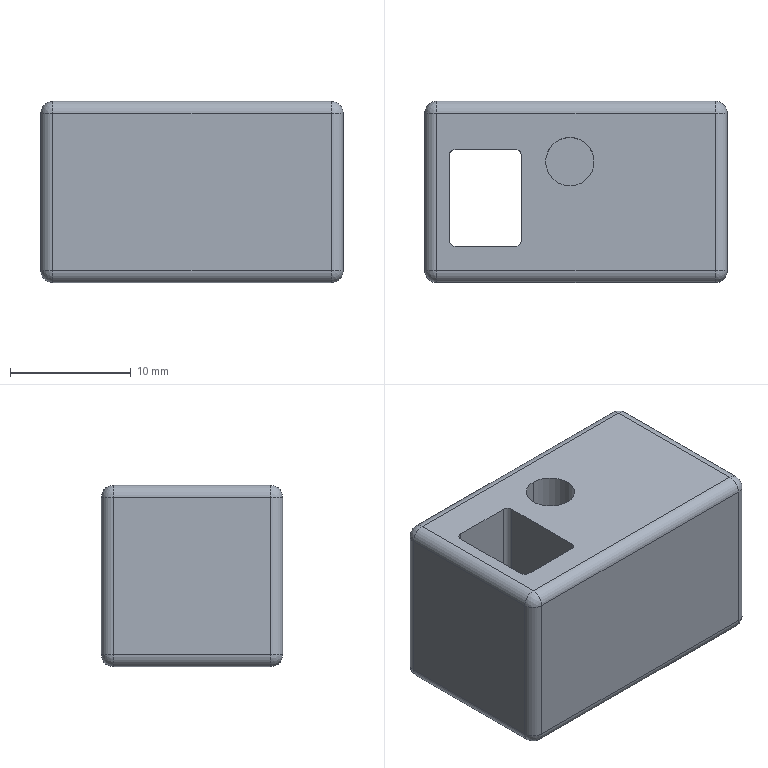Part | NX | 1 solid | 40 faces | box 25 x 15 x 15 mm | volume 4703 mm3 | cylinder 20 | plane 12 | sphere 8 | commonest cylinder face diameters 2 x12 1 x4 3.5 x2 4 x2
STEP:
#1=CARTESIAN_POINT('',(12.5,-6.5,-14.));
#2=VERTEX_POINT('',#1);
#3=CARTESIAN_POINT('',(12.5,6.5,-14.));
#4=VERTEX_POINT('',#3);
#5=CARTESIAN_POINT('',(12.5,-6.5,-14.));
#6=DIRECTION('',(0.,1.,0.));
#7=VECTOR('',#6,1000.);
#8=LINE('',#5,#7);
#9=EDGE_CURVE('',#2,#4,#8,.T.);
#10=ORIENTED_EDGE('',*,*,#9,.T.);
#11=CARTESIAN_POINT('',(12.5,6.5,-1.));
#12=VERTEX_POINT('',#11);
#13=CARTESIAN_POINT('',(12.5,6.5,-14.));
#14=DIRECTION('',(0.,0.,1.));
#15=VECTOR('',#14,1000.);
#16=LINE('',#13,#15);
#17=EDGE_CURVE('',#4,#12,#16,.T.);
#18=ORIENTED_EDGE('',*,*,#17,.T.);
#19=CARTESIAN_POINT('',(12.5,-6.5,-1.));
#20=VERTEX_POINT('',#19);
#21=CARTESIAN_POINT('',(12.5,6.5,-1.));
#22=DIRECTION('',(0.,-1.,0.));
#23=VECTOR('',#22,1000.);
#24=LINE('',#21,#23);
#25=EDGE_CURVE('',#12,#20,#24,.T.);
#26=ORIENTED_EDGE('',*,*,#25,.T.);
#27=CARTESIAN_POINT('',(12.5,-6.5,-1.));
#28=DIRECTION('',(0.,0.,-1.));
#29=VECTOR('',#28,1000.);
#30=LINE('',#27,#29);
#31=EDGE_CURVE('',#20,#2,#30,.T.);
#32=ORIENTED_EDGE('',*,*,#31,.T.);
#33=EDGE_LOOP('',(#10,#18,#26,#32));
#34=FACE_BOUND('',#33,.T.);
#35=CARTESIAN_POINT('',(12.5,0.75,-7.5));
#36=VERTEX_POINT('',#35);
#37=CARTESIAN_POINT('',(12.5,4.25,-7.5));
#38=VERTEX_POINT('',#37);
#39=CARTESIAN_POINT('',(12.5,2.5,-7.5));
#40=DIRECTION('',(1.,0.,0.));
#41=DIRECTION('',(0.,-1.,0.));
#42=AXIS2_PLACEMENT_3D('',#39,#40,#41);
#43=CIRCLE('',#42,1.75);
#44=EDGE_CURVE('',#36,#38,#43,.T.);
#45=ORIENTED_EDGE('',*,*,#44,.F.);
#46=CARTESIAN_POINT('',(12.5,2.5,-7.5));
#47=DIRECTION('',(1.,0.,0.));
#48=DIRECTION('',(0.,1.,0.));
#49=AXIS2_PLACEMENT_3D('',#46,#47,#48);
#50=CIRCLE('',#49,1.75);
#51=EDGE_CURVE('',#38,#36,#50,.T.);
#52=ORIENTED_EDGE('',*,*,#51,.F.);
#53=EDGE_LOOP('',(#45,#52));
#54=FACE_BOUND('',#53,.T.);
#55=CARTESIAN_POINT('',(12.5,-26.5,-53.));
#56=DIRECTION('',(-1.,0.,0.));
#57=DIRECTION('',(0.,1.,0.));
#58=AXIS2_PLACEMENT_3D('',#55,#56,#57);
#59=PLANE('',#58);
#60=ADVANCED_FACE('',(#34,#54),#59,.F.);
#61=CARTESIAN_POINT('',(2.5,0.75,-7.5));
#62=VERTEX_POINT('',#61);
#63=CARTESIAN_POINT('',(12.5,0.75,-7.5));
#64=DIRECTION('',(-1.,0.,0.));
#65=VECTOR('',#64,1000.);
#66=LINE('',#63,#65);
#67=EDGE_CURVE('',#36,#62,#66,.T.);
#68=ORIENTED_EDGE('',*,*,#67,.T.);
#69=CARTESIAN_POINT('',(2.5,4.25,-7.5));
#70=VERTEX_POINT('',#69);
#71=CARTESIAN_POINT('',(2.5,2.5,-7.5));
#72=DIRECTION('',(1.,0.,0.));
#73=DIRECTION('',(0.,1.,0.));
#74=AXIS2_PLACEMENT_3D('',#71,#72,#73);
#75=CIRCLE('',#74,1.75);
#76=EDGE_CURVE('',#70,#62,#75,.T.);
#77=ORIENTED_EDGE('',*,*,#76,.F.);
#78=CARTESIAN_POINT('',(12.5,4.25,-7.5));
#79=DIRECTION('',(-1.,0.,0.));
#80=VECTOR('',#79,1000.);
#81=LINE('',#78,#80);
#82=EDGE_CURVE('',#38,#70,#81,.T.);
#83=ORIENTED_EDGE('',*,*,#82,.F.);
#84=ORIENTED_EDGE('',*,*,#51,.T.);
#85=EDGE_LOOP('',(#68,#77,#83,#84));
#86=FACE_BOUND('',#85,.T.);
#87=CARTESIAN_POINT('',(12.5,2.5,-7.5));
#88=DIRECTION('',(1.,0.,0.));
#89=DIRECTION('',(0.,-1.,0.));
#90=AXIS2_PLACEMENT_3D('',#87,#88,#89);
#91=CYLINDRICAL_SURFACE('',#90,1.75);
#92=ADVANCED_FACE('',(#86),#91,.F.);
#93=ORIENTED_EDGE('',*,*,#82,.T.);
#94=CARTESIAN_POINT('',(2.5,2.5,-7.5));
#95=DIRECTION('',(1.,0.,0.));
#96=DIRECTION('',(0.,-1.,0.));
#97=AXIS2_PLACEMENT_3D('',#94,#95,#96);
#98=CIRCLE('',#97,1.75);
#99=EDGE_CURVE('',#62,#70,#98,.T.);
#100=ORIENTED_EDGE('',*,*,#99,.F.);
#101=ORIENTED_EDGE('',*,*,#67,.F.);
#102=ORIENTED_EDGE('',*,*,#44,.T.);
#103=EDGE_LOOP('',(#93,#100,#101,#102));
#104=FACE_BOUND('',#103,.T.);
#105=CARTESIAN_POINT('',(12.5,2.5,-7.5));
#106=DIRECTION('',(1.,0.,0.));
#107=DIRECTION('',(0.,-1.,0.));
#108=AXIS2_PLACEMENT_3D('',#105,#106,#107);
#109=CYLINDRICAL_SURFACE('',#108,1.75);
#110=ADVANCED_FACE('',(#104),#109,.F.);
#111=ORIENTED_EDGE('',*,*,#99,.T.);
#112=ORIENTED_EDGE('',*,*,#76,.T.);
#113=EDGE_LOOP('',(#111,#112));
#114=FACE_BOUND('',#113,.T.);
#115=CARTESIAN_POINT('',(2.5,-26.5,-53.));
#116=DIRECTION('',(1.,0.,0.));
#117=DIRECTION('',(0.,-1.,0.));
#118=AXIS2_PLACEMENT_3D('',#115,#116,#117);
#119=PLANE('',#118);
#120=ADVANCED_FACE('',(#114),#119,.T.);
#121=CARTESIAN_POINT('',(11.5,-7.5,-1.));
#122=VERTEX_POINT('',#121);
#123=CARTESIAN_POINT('',(11.5,-6.5,-1.));
#124=DIRECTION('',(0.,0.,-1.));
#125=DIRECTION('',(1.,0.,0.));
#126=AXIS2_PLACEMENT_3D('',#123,#124,#125);
#127=CIRCLE('',#126,1.);
#128=EDGE_CURVE('',#20,#122,#127,.T.);
#129=ORIENTED_EDGE('',*,*,#128,.T.);
#130=CARTESIAN_POINT('',(11.5,-7.5,-14.));
#131=VERTEX_POINT('',#130);
#132=CARTESIAN_POINT('',(11.5,-7.5,-1.));
#133=DIRECTION('',(0.,0.,-1.));
#134=VECTOR('',#133,1000.);
#135=LINE('',#132,#134);
#136=EDGE_CURVE('',#122,#131,#135,.T.);
#137=ORIENTED_EDGE('',*,*,#136,.T.);
#138=CARTESIAN_POINT('',(11.5,-6.5,-14.));
#139=DIRECTION('',(0.,0.,-1.));
#140=DIRECTION('',(1.,0.,0.));
#141=AXIS2_PLACEMENT_3D('',#138,#139,#140);
#142=CIRCLE('',#141,1.);
#143=EDGE_CURVE('',#2,#131,#142,.T.);
#144=ORIENTED_EDGE('',*,*,#143,.F.);
#145=ORIENTED_EDGE('',*,*,#31,.F.);
#146=EDGE_LOOP('',(#129,#137,#144,#145));
#147=FACE_BOUND('',#146,.T.);
#148=CARTESIAN_POINT('',(11.5,-6.5,-0.9345));
#149=DIRECTION('',(0.,0.,-1.));
#150=DIRECTION('',(-1.,0.,0.));
#151=AXIS2_PLACEMENT_3D('',#148,#149,#150);
#152=CYLINDRICAL_SURFACE('',#151,1.);
#153=ADVANCED_FACE('',(#147),#152,.T.);
#154=ORIENTED_EDGE('',*,*,#143,.T.);
#155=CARTESIAN_POINT('',(11.5,-6.5,-15.));
#156=VERTEX_POINT('',#155);
#157=CARTESIAN_POINT('',(11.5,-6.5,-14.));
#158=DIRECTION('',(-1.,0.,0.));
#159=DIRECTION('',(0.,0.,-1.));
#160=AXIS2_PLACEMENT_3D('',#157,#158,#159);
#161=CIRCLE('',#160,1.);
#162=EDGE_CURVE('',#156,#131,#161,.T.);
#163=ORIENTED_EDGE('',*,*,#162,.F.);
#164=CARTESIAN_POINT('',(11.5,-6.5,-14.));
#165=DIRECTION('',(0.,1.,0.));
#166=DIRECTION('',(1.,0.,0.));
#167=AXIS2_PLACEMENT_3D('',#164,#165,#166);
#168=CIRCLE('',#167,1.);
#169=EDGE_CURVE('',#2,#156,#168,.T.);
#170=ORIENTED_EDGE('',*,*,#169,.F.);
#171=EDGE_LOOP('',(#154,#163,#170));
#172=FACE_BOUND('',#171,.T.);
#173=CARTESIAN_POINT('',(11.5,-6.5,-14.));
#174=DIRECTION('',(0.7071,0.,0.7071));
#175=DIRECTION('',(-0.7071,0.,0.7071));
#176=AXIS2_PLACEMENT_3D('',#173,#174,#175);
#177=SPHERICAL_SURFACE('',#176,1.);
#178=ADVANCED_FACE('',(#172),#177,.T.);
#179=CARTESIAN_POINT('',(11.5,6.5,-15.));
#180=VERTEX_POINT('',#179);
#181=CARTESIAN_POINT('',(11.5,-6.5,-15.));
#182=DIRECTION('',(0.,1.,0.));
#183=VECTOR('',#182,1000.);
#184=LINE('',#181,#183);
#185=EDGE_CURVE('',#156,#180,#184,.T.);
#186=ORIENTED_EDGE('',*,*,#185,.T.);
#187=CARTESIAN_POINT('',(11.5,6.5,-14.));
#188=DIRECTION('',(0.,-1.,0.));
#189=DIRECTION('',(0.,0.,-1.));
#190=AXIS2_PLACEMENT_3D('',#187,#188,#189);
#191=CIRCLE('',#190,1.);
#192=EDGE_CURVE('',#180,#4,#191,.T.);
#193=ORIENTED_EDGE('',*,*,#192,.T.);
#194=ORIENTED_EDGE('',*,*,#9,.F.);
#195=ORIENTED_EDGE('',*,*,#169,.T.);
#196=EDGE_LOOP('',(#186,#193,#194,#195));
#197=FACE_BOUND('',#196,.T.);
#198=CARTESIAN_POINT('',(11.5,-11.591,-14.));
#199=DIRECTION('',(0.,1.,0.));
#200=DIRECTION('',(-1.,0.,0.));
#201=AXIS2_PLACEMENT_3D('',#198,#199,#200);
#202=CYLINDRICAL_SURFACE('',#201,1.);
#203=ADVANCED_FACE('',(#197),#202,.T.);
#204=CARTESIAN_POINT('',(11.5,7.5,-14.));
#205=VERTEX_POINT('',#204);
#206=CARTESIAN_POINT('',(11.5,6.5,-14.));
#207=DIRECTION('',(1.,0.,0.));
#208=DIRECTION('',(0.,0.,-1.));
#209=AXIS2_PLACEMENT_3D('',#206,#207,#208);
#210=CIRCLE('',#209,1.);
#211=EDGE_CURVE('',#180,#205,#210,.T.);
#212=ORIENTED_EDGE('',*,*,#211,.T.);
#213=CARTESIAN_POINT('',(11.5,6.5,-14.));
#214=DIRECTION('',(0.,0.,1.));
#215=DIRECTION('',(1.,0.,0.));
#216=AXIS2_PLACEMENT_3D('',#213,#214,#215);
#217=CIRCLE('',#216,1.);
#218=EDGE_CURVE('',#4,#205,#217,.T.);
#219=ORIENTED_EDGE('',*,*,#218,.F.);
#220=ORIENTED_EDGE('',*,*,#192,.F.);
#221=EDGE_LOOP('',(#212,#219,#220));
#222=FACE_BOUND('',#221,.T.);
#223=CARTESIAN_POINT('',(11.5,6.5,-14.));
#224=DIRECTION('',(-0.7071,0.,-0.7071));
#225=DIRECTION('',(-0.7071,0.,0.7071));
#226=AXIS2_PLACEMENT_3D('',#223,#224,#225);
#227=SPHERICAL_SURFACE('',#226,1.);
#228=ADVANCED_FACE('',(#222),#227,.T.);
#229=ORIENTED_EDGE('',*,*,#218,.T.);
#230=CARTESIAN_POINT('',(11.5,7.5,-1.));
#231=VERTEX_POINT('',#230);
#232=CARTESIAN_POINT('',(11.5,7.5,-14.));
#233=DIRECTION('',(0.,0.,1.));
#234=VECTOR('',#233,1000.);
#235=LINE('',#232,#234);
#236=EDGE_CURVE('',#205,#231,#235,.T.);
#237=ORIENTED_EDGE('',*,*,#236,.T.);
#238=CARTESIAN_POINT('',(11.5,6.5,-1.));
#239=DIRECTION('',(0.,0.,1.));
#240=DIRECTION('',(1.,0.,0.));
#241=AXIS2_PLACEMENT_3D('',#238,#239,#240);
#242=CIRCLE('',#241,1.);
#243=EDGE_CURVE('',#12,#231,#242,.T.);
#244=ORIENTED_EDGE('',*,*,#243,.F.);
#245=ORIENTED_EDGE('',*,*,#17,.F.);
#246=EDGE_LOOP('',(#229,#237,#244,#245));
#247=FACE_BOUND('',#246,.T.);
#248=CARTESIAN_POINT('',(11.5,6.5,-14.063));
#249=DIRECTION('',(0.,0.,1.));
#250=DIRECTION('',(-1.,0.,0.));
#251=AXIS2_PLACEMENT_3D('',#248,#249,#250);
#252=CYLINDRICAL_SURFACE('',#251,1.);
#253=ADVANCED_FACE('',(#247),#252,.T.);
#254=ORIENTED_EDGE('',*,*,#243,.T.);
#255=CARTESIAN_POINT('',(11.5,6.5,0.));
#256=VERTEX_POINT('',#255);
#257=CARTESIAN_POINT('',(11.5,6.5,-1.));
#258=DIRECTION('',(-1.,0.,0.));
#259=DIRECTION('',(0.,0.,1.));
#260=AXIS2_PLACEMENT_3D('',#257,#258,#259);
#261=CIRCLE('',#260,1.);
#262=EDGE_CURVE('',#256,#231,#261,.T.);
#263=ORIENTED_EDGE('',*,*,#262,.F.);
#264=CARTESIAN_POINT('',(11.5,6.5,-1.));
#265=DIRECTION('',(0.,-1.,0.));
#266=DIRECTION('',(1.,0.,0.));
#267=AXIS2_PLACEMENT_3D('',#264,#265,#266);
#268=CIRCLE('',#267,1.);
#269=EDGE_CURVE('',#12,#256,#268,.T.);
#270=ORIENTED_EDGE('',*,*,#269,.F.);
#271=EDGE_LOOP('',(#254,#263,#270));
#272=FACE_BOUND('',#271,.T.);
#273=CARTESIAN_POINT('',(11.5,6.5,-1.));
#274=DIRECTION('',(0.7071,0.,-0.7071));
#275=DIRECTION('',(-0.7071,0.,-0.7071));
#276=AXIS2_PLACEMENT_3D('',#273,#274,#275);
#277=SPHERICAL_SURFACE('',#276,1.);
#278=ADVANCED_FACE('',(#272),#277,.T.);
#279=ORIENTED_EDGE('',*,*,#25,.F.);
#280=ORIENTED_EDGE('',*,*,#269,.T.);
#281=CARTESIAN_POINT('',(11.5,-6.5,0.));
#282=VERTEX_POINT('',#281);
#283=CARTESIAN_POINT('',(11.5,6.5,0.));
#284=DIRECTION('',(0.,-1.,0.));
#285=VECTOR('',#284,1000.);
#286=LINE('',#283,#285);
#287=EDGE_CURVE('',#256,#282,#286,.T.);
#288=ORIENTED_EDGE('',*,*,#287,.T.);
#289=CARTESIAN_POINT('',(11.5,-6.5,-1.));
#290=DIRECTION('',(0.,1.,0.));
#291=DIRECTION('',(0.,0.,1.));
#292=AXIS2_PLACEMENT_3D('',#289,#290,#291);
#293=CIRCLE('',#292,1.);
#294=EDGE_CURVE('',#282,#20,#293,.T.);
#295=ORIENTED_EDGE('',*,*,#294,.T.);
#296=EDGE_LOOP('',(#279,#280,#288,#295));
#297=FACE_BOUND('',#296,.T.);
#298=CARTESIAN_POINT('',(11.5,16.591,-1.));
#299=DIRECTION('',(0.,-1.,0.));
#300=DIRECTION('',(-1.,0.,0.));
#301=AXIS2_PLACEMENT_3D('',#298,#299,#300);
#302=CYLINDRICAL_SURFACE('',#301,1.);
#303=ADVANCED_FACE('',(#297),#302,.T.);
#304=CARTESIAN_POINT('',(11.5,-6.5,-1.));
#305=DIRECTION('',(1.,0.,0.));
#306=DIRECTION('',(0.,0.,1.));
#307=AXIS2_PLACEMENT_3D('',#304,#305,#306);
#308=CIRCLE('',#307,1.);
#309=EDGE_CURVE('',#282,#122,#308,.T.);
#310=ORIENTED_EDGE('',*,*,#309,.T.);
#311=ORIENTED_EDGE('',*,*,#128,.F.);
#312=ORIENTED_EDGE('',*,*,#294,.F.);
#313=EDGE_LOOP('',(#310,#311,#312));
#314=FACE_BOUND('',#313,.T.);
#315=CARTESIAN_POINT('',(11.5,-6.5,-1.));
#316=DIRECTION('',(-0.7071,0.,0.7071));
#317=DIRECTION('',(-0.7071,0.,-0.7071));
#318=AXIS2_PLACEMENT_3D('',#315,#316,#317);
#319=SPHERICAL_SURFACE('',#318,1.);
#320=ADVANCED_FACE('',(#314),#319,.T.);
#321=CARTESIAN_POINT('',(-11.5,-6.5,0.));
#322=VERTEX_POINT('',#321);
#323=CARTESIAN_POINT('',(-11.5,-7.5,-1.));
#324=VERTEX_POINT('',#323);
#325=CARTESIAN_POINT('',(-11.5,-6.5,-1.));
#326=DIRECTION('',(1.,0.,0.));
#327=DIRECTION('',(0.,0.,1.));
#328=AXIS2_PLACEMENT_3D('',#325,#326,#327);
#329=CIRCLE('',#328,1.);
#330=EDGE_CURVE('',#322,#324,#329,.T.);
#331=ORIENTED_EDGE('',*,*,#330,.T.);
#332=CARTESIAN_POINT('',(-11.5,-7.5,-1.));
#333=DIRECTION('',(1.,0.,0.));
#334=VECTOR('',#333,1000.);
#335=LINE('',#332,#334);
#336=EDGE_CURVE('',#324,#122,#335,.T.);
#337=ORIENTED_EDGE('',*,*,#336,.T.);
#338=ORIENTED_EDGE('',*,*,#309,.F.);
#339=CARTESIAN_POINT('',(-11.5,-6.5,0.));
#340=DIRECTION('',(1.,0.,0.));
#341=VECTOR('',#340,1000.);
#342=LINE('',#339,#341);
#343=EDGE_CURVE('',#322,#282,#342,.T.);
#344=ORIENTED_EDGE('',*,*,#343,.F.);
#345=EDGE_LOOP('',(#331,#337,#338,#344));
#346=FACE_BOUND('',#345,.T.);
#347=CARTESIAN_POINT('',(-11.565,-6.5,-1.));
#348=DIRECTION('',(1.,0.,0.));
#349=DIRECTION('',(0.,0.,-1.));
#350=AXIS2_PLACEMENT_3D('',#347,#348,#349);
#351=CYLINDRICAL_SURFACE('',#350,1.);
#352=ADVANCED_FACE('',(#346),#351,.T.);
#353=ORIENTED_EDGE('',*,*,#287,.F.);
#354=CARTESIAN_POINT('',(-11.5,6.5,0.));
#355=VERTEX_POINT('',#354);
#356=CARTESIAN_POINT('',(11.5,6.5,0.));
#357=DIRECTION('',(-1.,0.,0.));
#358=VECTOR('',#357,1000.);
#359=LINE('',#356,#358);
#360=EDGE_CURVE('',#256,#355,#359,.T.);
#361=ORIENTED_EDGE('',*,*,#360,.T.);
#362=CARTESIAN_POINT('',(-11.5,-6.5,0.));
#363=DIRECTION('',(0.,1.,0.));
#364=VECTOR('',#363,1000.);
#365=LINE('',#362,#364);
#366=EDGE_CURVE('',#322,#355,#365,.T.);
#367=ORIENTED_EDGE('',*,*,#366,.F.);
#368=ORIENTED_EDGE('',*,*,#343,.T.);
#369=EDGE_LOOP('',(#353,#361,#367,#368));
#370=FACE_BOUND('',#369,.T.);
#371=CARTESIAN_POINT('',(-0.5,0.5,0.));
#372=VERTEX_POINT('',#371);
#373=CARTESIAN_POINT('',(-0.5,4.5,0.));
#374=VERTEX_POINT('',#373);
#375=CARTESIAN_POINT('',(-0.5,2.5,0.));
#376=DIRECTION('',(0.,0.,1.));
#377=DIRECTION('',(0.,-1.,0.));
#378=AXIS2_PLACEMENT_3D('',#375,#376,#377);
#379=CIRCLE('',#378,2.);
#380=EDGE_CURVE('',#372,#374,#379,.T.);
#381=ORIENTED_EDGE('',*,*,#380,.F.);
#382=CARTESIAN_POINT('',(-0.5,2.5,0.));
#383=DIRECTION('',(0.,0.,1.));
#384=DIRECTION('',(0.,1.,0.));
#385=AXIS2_PLACEMENT_3D('',#382,#383,#384);
#386=CIRCLE('',#385,2.);
#387=EDGE_CURVE('',#374,#372,#386,.T.);
#388=ORIENTED_EDGE('',*,*,#387,.F.);
#389=EDGE_LOOP('',(#381,#388));
#390=FACE_BOUND('',#389,.T.);
#391=CARTESIAN_POINT('',(-10.,-4.5,0.));
#392=VERTEX_POINT('',#391);
#393=CARTESIAN_POINT('',(-10.5,-4.,0.));
#394=VERTEX_POINT('',#393);
#395=CARTESIAN_POINT('',(-10.,-4.,0.));
#396=DIRECTION('',(0.,0.,-1.));
#397=DIRECTION('',(0.,-1.,0.));
#398=AXIS2_PLACEMENT_3D('',#395,#396,#397);
#399=CIRCLE('',#398,0.5);
#400=EDGE_CURVE('',#392,#394,#399,.T.);
#401=ORIENTED_EDGE('',*,*,#400,.T.);
#402=CARTESIAN_POINT('',(-10.5,3.,0.));
#403=VERTEX_POINT('',#402);
#404=CARTESIAN_POINT('',(-10.5,-4.,0.));
#405=DIRECTION('',(0.,1.,0.));
#406=VECTOR('',#405,1000.);
#407=LINE('',#404,#406);
#408=EDGE_CURVE('',#394,#403,#407,.T.);
#409=ORIENTED_EDGE('',*,*,#408,.T.);
#410=CARTESIAN_POINT('',(-10.,3.5,0.));
#411=VERTEX_POINT('',#410);
#412=CARTESIAN_POINT('',(-10.,3.,0.));
#413=DIRECTION('',(0.,0.,-1.));
#414=DIRECTION('',(-1.,0.,0.));
#415=AXIS2_PLACEMENT_3D('',#412,#413,#414);
#416=CIRCLE('',#415,0.5);
#417=EDGE_CURVE('',#403,#411,#416,.T.);
#418=ORIENTED_EDGE('',*,*,#417,.T.);
#419=CARTESIAN_POINT('',(-5.,3.5,0.));
#420=VERTEX_POINT('',#419);
#421=CARTESIAN_POINT('',(-10.,3.5,0.));
#422=DIRECTION('',(1.,0.,0.));
#423=VECTOR('',#422,1000.);
#424=LINE('',#421,#423);
#425=EDGE_CURVE('',#411,#420,#424,.T.);
#426=ORIENTED_EDGE('',*,*,#425,.T.);
#427=CARTESIAN_POINT('',(-4.5,3.,0.));
#428=VERTEX_POINT('',#427);
#429=CARTESIAN_POINT('',(-5.,3.,0.));
#430=DIRECTION('',(0.,0.,-1.));
#431=DIRECTION('',(0.,1.,0.));
#432=AXIS2_PLACEMENT_3D('',#429,#430,#431);
#433=CIRCLE('',#432,0.5);
#434=EDGE_CURVE('',#420,#428,#433,.T.);
#435=ORIENTED_EDGE('',*,*,#434,.T.);
#436=CARTESIAN_POINT('',(-4.5,-4.,0.));
#437=VERTEX_POINT('',#436);
#438=CARTESIAN_POINT('',(-4.5,3.,0.));
#439=DIRECTION('',(0.,-1.,0.));
#440=VECTOR('',#439,1000.);
#441=LINE('',#438,#440);
#442=EDGE_CURVE('',#428,#437,#441,.T.);
#443=ORIENTED_EDGE('',*,*,#442,.T.);
#444=CARTESIAN_POINT('',(-5.,-4.5,0.));
#445=VERTEX_POINT('',#444);
#446=CARTESIAN_POINT('',(-5.,-4.,0.));
#447=DIRECTION('',(0.,0.,-1.));
#448=DIRECTION('',(1.,0.,0.));
#449=AXIS2_PLACEMENT_3D('',#446,#447,#448);
#450=CIRCLE('',#449,0.5);
#451=EDGE_CURVE('',#437,#445,#450,.T.);
#452=ORIENTED_EDGE('',*,*,#451,.T.);
#453=CARTESIAN_POINT('',(-5.,-4.5,0.));
#454=DIRECTION('',(-1.,0.,0.));
#455=VECTOR('',#454,1000.);
#456=LINE('',#453,#455);
#457=EDGE_CURVE('',#445,#392,#456,.T.);
#458=ORIENTED_EDGE('',*,*,#457,.T.);
#459=EDGE_LOOP('',(#401,#409,#418,#426,#435,#443,#452,#458));
#460=FACE_BOUND('',#459,.T.);
#461=CARTESIAN_POINT('',(12.5,-12.5,0.));
#462=DIRECTION('',(0.,0.,1.));
#463=DIRECTION('',(0.,-1.,0.));
#464=AXIS2_PLACEMENT_3D('',#461,#462,#463);
#465=PLANE('',#464);
#466=ADVANCED_FACE('',(#370,#390,#460),#465,.T.);
#467=ORIENTED_EDGE('',*,*,#457,.F.);
#468=CARTESIAN_POINT('',(-5.,-4.5,-15.));
#469=VERTEX_POINT('',#468);
#470=CARTESIAN_POINT('',(-5.,-4.5,-15.));
#471=DIRECTION('',(0.,0.,1.));
#472=VECTOR('',#471,1000.);
#473=LINE('',#470,#472);
#474=EDGE_CURVE('',#469,#445,#473,.T.);
#475=ORIENTED_EDGE('',*,*,#474,.F.);
#476=CARTESIAN_POINT('',(-10.,-4.5,-15.));
#477=VERTEX_POINT('',#476);
#478=CARTESIAN_POINT('',(-5.,-4.5,-15.));
#479=DIRECTION('',(-1.,0.,0.));
#480=VECTOR('',#479,1000.);
#481=LINE('',#478,#480);
#482=EDGE_CURVE('',#469,#477,#481,.T.);
#483=ORIENTED_EDGE('',*,*,#482,.T.);
#484=CARTESIAN_POINT('',(-10.,-4.5,0.));
#485=DIRECTION('',(0.,0.,-1.));
#486=VECTOR('',#485,1000.);
#487=LINE('',#484,#486);
#488=EDGE_CURVE('',#392,#477,#487,.T.);
#489=ORIENTED_EDGE('',*,*,#488,.F.);
#490=EDGE_LOOP('',(#467,#475,#483,#489));
#491=FACE_BOUND('',#490,.T.);
#492=CARTESIAN_POINT('',(-2.5,-4.5,0.));
#493=DIRECTION('',(0.,1.,0.));
#494=DIRECTION('',(1.,0.,0.));
#495=AXIS2_PLACEMENT_3D('',#492,#493,#494);
#496=PLANE('',#495);
#497=ADVANCED_FACE('',(#491),#496,.T.);
#498=CARTESIAN_POINT('',(-10.5,-4.,-15.));
#499=VERTEX_POINT('',#498);
#500=CARTESIAN_POINT('',(-10.,-4.,-15.));
#501=DIRECTION('',(0.,0.,1.));
#502=DIRECTION('',(-1.,0.,0.));
#503=AXIS2_PLACEMENT_3D('',#500,#501,#502);
#504=CIRCLE('',#503,0.5);
#505=EDGE_CURVE('',#499,#477,#504,.T.);
#506=ORIENTED_EDGE('',*,*,#505,.F.);
#507=CARTESIAN_POINT('',(-10.5,-4.,0.));
#508=DIRECTION('',(0.,0.,-1.));
#509=VECTOR('',#508,1000.);
#510=LINE('',#507,#509);
#511=EDGE_CURVE('',#394,#499,#510,.T.);
#512=ORIENTED_EDGE('',*,*,#511,.F.);
#513=ORIENTED_EDGE('',*,*,#400,.F.);
#514=ORIENTED_EDGE('',*,*,#488,.T.);
#515=EDGE_LOOP('',(#506,#512,#513,#514));
#516=FACE_BOUND('',#515,.T.);
#517=CARTESIAN_POINT('',(-10.,-4.,19.554));
#518=DIRECTION('',(0.,0.,-1.));
#519=DIRECTION('',(0.,1.,0.));
#520=AXIS2_PLACEMENT_3D('',#517,#518,#519);
#521=CYLINDRICAL_SURFACE('',#520,0.5);
#522=ADVANCED_FACE('',(#516),#521,.F.);
#523=CARTESIAN_POINT('',(-10.5,3.,-15.));
#524=VERTEX_POINT('',#523);
#525=CARTESIAN_POINT('',(-10.5,-4.,-15.));
#526=DIRECTION('',(0.,1.,0.));
#527=VECTOR('',#526,1000.);
#528=LINE('',#525,#527);
#529=EDGE_CURVE('',#499,#524,#528,.T.);
#530=ORIENTED_EDGE('',*,*,#529,.T.);
#531=CARTESIAN_POINT('',(-10.5,3.,-15.));
#532=DIRECTION('',(0.,0.,1.));
#533=VECTOR('',#532,1000.);
#534=LINE('',#531,#533);
#535=EDGE_CURVE('',#524,#403,#534,.T.);
#536=ORIENTED_EDGE('',*,*,#535,.T.);
#537=ORIENTED_EDGE('',*,*,#408,.F.);
#538=ORIENTED_EDGE('',*,*,#511,.T.);
#539=EDGE_LOOP('',(#530,#536,#537,#538));
#540=FACE_BOUND('',#539,.T.);
#541=CARTESIAN_POINT('',(-10.5,-4.5,0.));
#542=DIRECTION('',(1.,0.,0.));
#543=DIRECTION('',(0.,-1.,0.));
#544=AXIS2_PLACEMENT_3D('',#541,#542,#543);
#545=PLANE('',#544);
#546=ADVANCED_FACE('',(#540),#545,.T.);
#547=ORIENTED_EDGE('',*,*,#417,.F.);
#548=ORIENTED_EDGE('',*,*,#535,.F.);
#549=CARTESIAN_POINT('',(-10.,3.5,-15.));
#550=VERTEX_POINT('',#549);
#551=CARTESIAN_POINT('',(-10.,3.,-15.));
#552=DIRECTION('',(0.,0.,1.));
#553=DIRECTION('',(0.,1.,0.));
#554=AXIS2_PLACEMENT_3D('',#551,#552,#553);
#555=CIRCLE('',#554,0.5);
#556=EDGE_CURVE('',#550,#524,#555,.T.);
#557=ORIENTED_EDGE('',*,*,#556,.F.);
#558=CARTESIAN_POINT('',(-10.,3.5,-15.));
#559=DIRECTION('',(0.,0.,1.));
#560=VECTOR('',#559,1000.);
#561=LINE('',#558,#560);
#562=EDGE_CURVE('',#550,#411,#561,.T.);
#563=ORIENTED_EDGE('',*,*,#562,.T.);
#564=EDGE_LOOP('',(#547,#548,#557,#563));
#565=FACE_BOUND('',#564,.T.);
#566=CARTESIAN_POINT('',(-10.,3.,-34.554));
#567=DIRECTION('',(0.,0.,1.));
#568=DIRECTION('',(0.,-1.,0.));
#569=AXIS2_PLACEMENT_3D('',#566,#567,#568);
#570=CYLINDRICAL_SURFACE('',#569,0.5);
#571=ADVANCED_FACE('',(#565),#570,.F.);
#572=ORIENTED_EDGE('',*,*,#425,.F.);
#573=ORIENTED_EDGE('',*,*,#562,.F.);
#574=CARTESIAN_POINT('',(-5.,3.5,-15.));
#575=VERTEX_POINT('',#574);
#576=CARTESIAN_POINT('',(-10.,3.5,-15.));
#577=DIRECTION('',(1.,0.,0.));
#578=VECTOR('',#577,1000.);
#579=LINE('',#576,#578);
#580=EDGE_CURVE('',#550,#575,#579,.T.);
#581=ORIENTED_EDGE('',*,*,#580,.T.);
#582=CARTESIAN_POINT('',(-5.,3.5,-15.));
#583=DIRECTION('',(0.,0.,1.));
#584=VECTOR('',#583,1000.);
#585=LINE('',#582,#584);
#586=EDGE_CURVE('',#575,#420,#585,.T.);
#587=ORIENTED_EDGE('',*,*,#586,.T.);
#588=EDGE_LOOP('',(#572,#573,#581,#587));
#589=FACE_BOUND('',#588,.T.);
#590=CARTESIAN_POINT('',(-10.5,3.5,0.));
#591=DIRECTION('',(0.,-1.,0.));
#592=DIRECTION('',(-1.,0.,0.));
#593=AXIS2_PLACEMENT_3D('',#590,#591,#592);
#594=PLANE('',#593);
#595=ADVANCED_FACE('',(#589),#594,.T.);
#596=ORIENTED_EDGE('',*,*,#434,.F.);
#597=ORIENTED_EDGE('',*,*,#586,.F.);
#598=CARTESIAN_POINT('',(-4.5,3.,-15.));
#599=VERTEX_POINT('',#598);
#600=CARTESIAN_POINT('',(-5.,3.,-15.));
#601=DIRECTION('',(0.,0.,1.));
#602=DIRECTION('',(1.,0.,0.));
#603=AXIS2_PLACEMENT_3D('',#600,#601,#602);
#604=CIRCLE('',#603,0.5);
#605=EDGE_CURVE('',#599,#575,#604,.T.);
#606=ORIENTED_EDGE('',*,*,#605,.F.);
#607=CARTESIAN_POINT('',(-4.5,3.,-15.));
#608=DIRECTION('',(0.,0.,1.));
#609=VECTOR('',#608,1000.);
#610=LINE('',#607,#609);
#611=EDGE_CURVE('',#599,#428,#610,.T.);
#612=ORIENTED_EDGE('',*,*,#611,.T.);
#613=EDGE_LOOP('',(#596,#597,#606,#612));
#614=FACE_BOUND('',#613,.T.);
#615=CARTESIAN_POINT('',(-5.,3.,-34.554));
#616=DIRECTION('',(0.,0.,1.));
#617=DIRECTION('',(-1.,0.,0.));
#618=AXIS2_PLACEMENT_3D('',#615,#616,#617);
#619=CYLINDRICAL_SURFACE('',#618,0.5);
#620=ADVANCED_FACE('',(#614),#619,.F.);
#621=ORIENTED_EDGE('',*,*,#442,.F.);
#622=ORIENTED_EDGE('',*,*,#611,.F.);
#623=CARTESIAN_POINT('',(-4.5,-4.,-15.));
#624=VERTEX_POINT('',#623);
#625=CARTESIAN_POINT('',(-4.5,3.,-15.));
#626=DIRECTION('',(0.,-1.,0.));
#627=VECTOR('',#626,1000.);
#628=LINE('',#625,#627);
#629=EDGE_CURVE('',#599,#624,#628,.T.);
#630=ORIENTED_EDGE('',*,*,#629,.T.);
#631=CARTESIAN_POINT('',(-4.5,-4.,-15.));
#632=DIRECTION('',(0.,0.,1.));
#633=VECTOR('',#632,1000.);
#634=LINE('',#631,#633);
#635=EDGE_CURVE('',#624,#437,#634,.T.);
#636=ORIENTED_EDGE('',*,*,#635,.T.);
#637=EDGE_LOOP('',(#621,#622,#630,#636));
#638=FACE_BOUND('',#637,.T.);
#639=CARTESIAN_POINT('',(-4.5,3.5,0.));
#640=DIRECTION('',(-1.,0.,0.));
#641=DIRECTION('',(0.,1.,0.));
#642=AXIS2_PLACEMENT_3D('',#639,#640,#641);
#643=PLANE('',#642);
#644=ADVANCED_FACE('',(#638),#643,.T.);
#645=ORIENTED_EDGE('',*,*,#451,.F.);
#646=ORIENTED_EDGE('',*,*,#635,.F.);
#647=CARTESIAN_POINT('',(-5.,-4.,-15.));
#648=DIRECTION('',(0.,0.,1.));
#649=DIRECTION('',(0.,-1.,0.));
#650=AXIS2_PLACEMENT_3D('',#647,#648,#649);
#651=CIRCLE('',#650,0.5);
#652=EDGE_CURVE('',#469,#624,#651,.T.);
#653=ORIENTED_EDGE('',*,*,#652,.F.);
#654=ORIENTED_EDGE('',*,*,#474,.T.);
#655=EDGE_LOOP('',(#645,#646,#653,#654));
#656=FACE_BOUND('',#655,.T.);
#657=CARTESIAN_POINT('',(-5.,-4.,-34.554));
#658=DIRECTION('',(0.,0.,1.));
#659=DIRECTION('',(0.,1.,0.));
#660=AXIS2_PLACEMENT_3D('',#657,#658,#659);
#661=CYLINDRICAL_SURFACE('',#660,0.5);
#662=ADVANCED_FACE('',(#656),#661,.F.);
#663=CARTESIAN_POINT('',(-11.5,6.5,-15.));
#664=VERTEX_POINT('',#663);
#665=CARTESIAN_POINT('',(-11.5,-6.5,-15.));
#666=VERTEX_POINT('',#665);
#667=CARTESIAN_POINT('',(-11.5,6.5,-15.));
#668=DIRECTION('',(0.,-1.,0.));
#669=VECTOR('',#668,1000.);
#670=LINE('',#667,#669);
#671=EDGE_CURVE('',#664,#666,#670,.T.);
#672=ORIENTED_EDGE('',*,*,#671,.F.);
#673=CARTESIAN_POINT('',(-11.5,6.5,-15.));
#674=DIRECTION('',(1.,0.,0.));
#675=VECTOR('',#674,1000.);
#676=LINE('',#673,#675);
#677=EDGE_CURVE('',#664,#180,#676,.T.);
#678=ORIENTED_EDGE('',*,*,#677,.T.);
#679=ORIENTED_EDGE('',*,*,#185,.F.);
#680=CARTESIAN_POINT('',(11.5,-6.5,-15.));
#681=DIRECTION('',(-1.,0.,0.));
#682=VECTOR('',#681,1000.);
#683=LINE('',#680,#682);
#684=EDGE_CURVE('',#156,#666,#683,.T.);
#685=ORIENTED_EDGE('',*,*,#684,.T.);
#686=EDGE_LOOP('',(#672,#678,#679,#685));
#687=FACE_BOUND('',#686,.T.);
#688=ORIENTED_EDGE('',*,*,#605,.T.);
#689=ORIENTED_EDGE('',*,*,#580,.F.);
#690=ORIENTED_EDGE('',*,*,#556,.T.);
#691=ORIENTED_EDGE('',*,*,#529,.F.);
#692=ORIENTED_EDGE('',*,*,#505,.T.);
#693=ORIENTED_EDGE('',*,*,#482,.F.);
#694=ORIENTED_EDGE('',*,*,#652,.T.);
#695=ORIENTED_EDGE('',*,*,#629,.F.);
#696=EDGE_LOOP('',(#688,#689,#690,#691,#692,#693,#694,#695));
#697=FACE_BOUND('',#696,.T.);
#698=CARTESIAN_POINT('',(12.5,17.5,-15.));
#699=DIRECTION('',(0.,0.,-1.));
#700=DIRECTION('',(0.,1.,0.));
#701=AXIS2_PLACEMENT_3D('',#698,#699,#700);
#702=PLANE('',#701);
#703=ADVANCED_FACE('',(#687,#697),#702,.T.);
#704=ORIENTED_EDGE('',*,*,#162,.T.);
#705=CARTESIAN_POINT('',(-11.5,-7.5,-14.));
#706=VERTEX_POINT('',#705);
#707=CARTESIAN_POINT('',(11.5,-7.5,-14.));
#708=DIRECTION('',(-1.,0.,0.));
#709=VECTOR('',#708,1000.);
#710=LINE('',#707,#709);
#711=EDGE_CURVE('',#131,#706,#710,.T.);
#712=ORIENTED_EDGE('',*,*,#711,.T.);
#713=CARTESIAN_POINT('',(-11.5,-6.5,-14.));
#714=DIRECTION('',(-1.,0.,0.));
#715=DIRECTION('',(0.,0.,-1.));
#716=AXIS2_PLACEMENT_3D('',#713,#714,#715);
#717=CIRCLE('',#716,1.);
#718=EDGE_CURVE('',#666,#706,#717,.T.);
#719=ORIENTED_EDGE('',*,*,#718,.F.);
#720=ORIENTED_EDGE('',*,*,#684,.F.);
#721=EDGE_LOOP('',(#704,#712,#719,#720));
#722=FACE_BOUND('',#721,.T.);
#723=CARTESIAN_POINT('',(11.563,-6.5,-14.));
#724=DIRECTION('',(-1.,0.,0.));
#725=DIRECTION('',(0.,0.,1.));
#726=AXIS2_PLACEMENT_3D('',#723,#724,#725);
#727=CYLINDRICAL_SURFACE('',#726,1.);
#728=ADVANCED_FACE('',(#722),#727,.T.);
#729=ORIENTED_EDGE('',*,*,#718,.T.);
#730=CARTESIAN_POINT('',(-12.5,-6.5,-14.));
#731=VERTEX_POINT('',#730);
#732=CARTESIAN_POINT('',(-11.5,-6.5,-14.));
#733=DIRECTION('',(0.,0.,1.));
#734=DIRECTION('',(-1.,0.,0.));
#735=AXIS2_PLACEMENT_3D('',#732,#733,#734);
#736=CIRCLE('',#735,1.);
#737=EDGE_CURVE('',#731,#706,#736,.T.);
#738=ORIENTED_EDGE('',*,*,#737,.F.);
#739=CARTESIAN_POINT('',(-11.5,-6.5,-14.));
#740=DIRECTION('',(0.,1.,0.));
#741=DIRECTION('',(0.,0.,-1.));
#742=AXIS2_PLACEMENT_3D('',#739,#740,#741);
#743=CIRCLE('',#742,1.);
#744=EDGE_CURVE('',#666,#731,#743,.T.);
#745=ORIENTED_EDGE('',*,*,#744,.F.);
#746=EDGE_LOOP('',(#729,#738,#745));
#747=FACE_BOUND('',#746,.T.);
#748=CARTESIAN_POINT('',(-11.5,-6.5,-14.));
#749=DIRECTION('',(0.7071,0.,-0.7071));
#750=DIRECTION('',(0.7071,0.,0.7071));
#751=AXIS2_PLACEMENT_3D('',#748,#749,#750);
#752=SPHERICAL_SURFACE('',#751,1.);
#753=ADVANCED_FACE('',(#747),#752,.T.);
#754=CARTESIAN_POINT('',(-12.5,6.5,-14.));
#755=VERTEX_POINT('',#754);
#756=CARTESIAN_POINT('',(-12.5,6.5,-14.));
#757=DIRECTION('',(0.,-1.,0.));
#758=VECTOR('',#757,1000.);
#759=LINE('',#756,#758);
#760=EDGE_CURVE('',#755,#731,#759,.T.);
#761=ORIENTED_EDGE('',*,*,#760,.F.);
#762=CARTESIAN_POINT('',(-11.5,6.5,-14.));
#763=DIRECTION('',(0.,-1.,0.));
#764=DIRECTION('',(-1.,0.,0.));
#765=AXIS2_PLACEMENT_3D('',#762,#763,#764);
#766=CIRCLE('',#765,1.);
#767=EDGE_CURVE('',#755,#664,#766,.T.);
#768=ORIENTED_EDGE('',*,*,#767,.T.);
#769=ORIENTED_EDGE('',*,*,#671,.T.);
#770=ORIENTED_EDGE('',*,*,#744,.T.);
#771=EDGE_LOOP('',(#761,#768,#769,#770));
#772=FACE_BOUND('',#771,.T.);
#773=CARTESIAN_POINT('',(-11.5,16.564,-14.));
#774=DIRECTION('',(0.,-1.,0.));
#775=DIRECTION('',(1.,0.,0.));
#776=AXIS2_PLACEMENT_3D('',#773,#774,#775);
#777=CYLINDRICAL_SURFACE('',#776,1.);
#778=ADVANCED_FACE('',(#772),#777,.T.);
#779=CARTESIAN_POINT('',(-11.5,7.5,-14.));
#780=VERTEX_POINT('',#779);
#781=CARTESIAN_POINT('',(-11.5,6.5,-14.));
#782=DIRECTION('',(0.,0.,-1.));
#783=DIRECTION('',(-1.,0.,0.));
#784=AXIS2_PLACEMENT_3D('',#781,#782,#783);
#785=CIRCLE('',#784,1.);
#786=EDGE_CURVE('',#755,#780,#785,.T.);
#787=ORIENTED_EDGE('',*,*,#786,.T.);
#788=CARTESIAN_POINT('',(-11.5,6.5,-14.));
#789=DIRECTION('',(1.,0.,0.));
#790=DIRECTION('',(0.,0.,-1.));
#791=AXIS2_PLACEMENT_3D('',#788,#789,#790);
#792=CIRCLE('',#791,1.);
#793=EDGE_CURVE('',#664,#780,#792,.T.);
#794=ORIENTED_EDGE('',*,*,#793,.F.);
#795=ORIENTED_EDGE('',*,*,#767,.F.);
#796=EDGE_LOOP('',(#787,#794,#795));
#797=FACE_BOUND('',#796,.T.);
#798=CARTESIAN_POINT('',(-11.5,6.5,-14.));
#799=DIRECTION('',(-0.7071,0.,0.7071));
#800=DIRECTION('',(0.7071,0.,0.7071));
#801=AXIS2_PLACEMENT_3D('',#798,#799,#800);
#802=SPHERICAL_SURFACE('',#801,1.);
#803=ADVANCED_FACE('',(#797),#802,.T.);
#804=ORIENTED_EDGE('',*,*,#793,.T.);
#805=CARTESIAN_POINT('',(-11.5,7.5,-14.));
#806=DIRECTION('',(1.,0.,0.));
#807=VECTOR('',#806,1000.);
#808=LINE('',#805,#807);
#809=EDGE_CURVE('',#780,#205,#808,.T.);
#810=ORIENTED_EDGE('',*,*,#809,.T.);
#811=ORIENTED_EDGE('',*,*,#211,.F.);
#812=ORIENTED_EDGE('',*,*,#677,.F.);
#813=EDGE_LOOP('',(#804,#810,#811,#812));
#814=FACE_BOUND('',#813,.T.);
#815=CARTESIAN_POINT('',(-11.565,6.5,-14.));
#816=DIRECTION('',(1.,0.,0.));
#817=DIRECTION('',(0.,0.,1.));
#818=AXIS2_PLACEMENT_3D('',#815,#816,#817);
#819=CYLINDRICAL_SURFACE('',#818,1.);
#820=ADVANCED_FACE('',(#814),#819,.T.);
#821=CARTESIAN_POINT('',(-11.5,7.5,-1.));
#822=VERTEX_POINT('',#821);
#823=CARTESIAN_POINT('',(11.5,7.5,-1.));
#824=DIRECTION('',(-1.,0.,0.));
#825=VECTOR('',#824,1000.);
#826=LINE('',#823,#825);
#827=EDGE_CURVE('',#231,#822,#826,.T.);
#828=ORIENTED_EDGE('',*,*,#827,.F.);
#829=ORIENTED_EDGE('',*,*,#236,.F.);
#830=ORIENTED_EDGE('',*,*,#809,.F.);
#831=CARTESIAN_POINT('',(-11.5,7.5,-1.));
#832=DIRECTION('',(0.,0.,-1.));
#833=VECTOR('',#832,1000.);
#834=LINE('',#831,#833);
#835=EDGE_CURVE('',#822,#780,#834,.T.);
#836=ORIENTED_EDGE('',*,*,#835,.F.);
#837=EDGE_LOOP('',(#828,#829,#830,#836));
#838=FACE_BOUND('',#837,.T.);
#839=CARTESIAN_POINT('',(-12.5,7.5,-15.));
#840=DIRECTION('',(0.,-1.,0.));
#841=DIRECTION('',(0.,0.,-1.));
#842=AXIS2_PLACEMENT_3D('',#839,#840,#841);
#843=PLANE('',#842);
#844=ADVANCED_FACE('',(#838),#843,.F.);
#845=CARTESIAN_POINT('',(-12.5,6.5,-1.));
#846=VERTEX_POINT('',#845);
#847=CARTESIAN_POINT('',(-11.5,6.5,-1.));
#848=DIRECTION('',(0.,0.,-1.));
#849=DIRECTION('',(-1.,0.,0.));
#850=AXIS2_PLACEMENT_3D('',#847,#848,#849);
#851=CIRCLE('',#850,1.);
#852=EDGE_CURVE('',#846,#822,#851,.T.);
#853=ORIENTED_EDGE('',*,*,#852,.T.);
#854=ORIENTED_EDGE('',*,*,#835,.T.);
#855=ORIENTED_EDGE('',*,*,#786,.F.);
#856=CARTESIAN_POINT('',(-12.5,6.5,-1.));
#857=DIRECTION('',(0.,0.,-1.));
#858=VECTOR('',#857,1000.);
#859=LINE('',#856,#858);
#860=EDGE_CURVE('',#846,#755,#859,.T.);
#861=ORIENTED_EDGE('',*,*,#860,.F.);
#862=EDGE_LOOP('',(#853,#854,#855,#861));
#863=FACE_BOUND('',#862,.T.);
#864=CARTESIAN_POINT('',(-11.5,6.5,-0.9345));
#865=DIRECTION('',(0.,0.,-1.));
#866=DIRECTION('',(1.,0.,0.));
#867=AXIS2_PLACEMENT_3D('',#864,#865,#866);
#868=CYLINDRICAL_SURFACE('',#867,1.);
#869=ADVANCED_FACE('',(#863),#868,.T.);
#870=CARTESIAN_POINT('',(-12.5,-6.5,-1.));
#871=VERTEX_POINT('',#870);
#872=CARTESIAN_POINT('',(-12.5,-6.5,-1.));
#873=DIRECTION('',(0.,1.,0.));
#874=VECTOR('',#873,1000.);
#875=LINE('',#872,#874);
#876=EDGE_CURVE('',#871,#846,#875,.T.);
#877=ORIENTED_EDGE('',*,*,#876,.T.);
#878=ORIENTED_EDGE('',*,*,#860,.T.);
#879=ORIENTED_EDGE('',*,*,#760,.T.);
#880=CARTESIAN_POINT('',(-12.5,-6.5,-14.));
#881=DIRECTION('',(0.,0.,1.));
#882=VECTOR('',#881,1000.);
#883=LINE('',#880,#882);
#884=EDGE_CURVE('',#731,#871,#883,.T.);
#885=ORIENTED_EDGE('',*,*,#884,.T.);
#886=EDGE_LOOP('',(#877,#878,#879,#885));
#887=FACE_BOUND('',#886,.T.);
#888=CARTESIAN_POINT('',(-12.5,-4.5,0.));
#889=DIRECTION('',(-1.,0.,0.));
#890=DIRECTION('',(0.,1.,0.));
#891=AXIS2_PLACEMENT_3D('',#888,#889,#890);
#892=PLANE('',#891);
#893=ADVANCED_FACE('',(#887),#892,.T.);
#894=ORIENTED_EDGE('',*,*,#737,.T.);
#895=CARTESIAN_POINT('',(-11.5,-7.5,-14.));
#896=DIRECTION('',(0.,0.,1.));
#897=VECTOR('',#896,1000.);
#898=LINE('',#895,#897);
#899=EDGE_CURVE('',#706,#324,#898,.T.);
#900=ORIENTED_EDGE('',*,*,#899,.T.);
#901=CARTESIAN_POINT('',(-11.5,-6.5,-1.));
#902=DIRECTION('',(0.,0.,1.));
#903=DIRECTION('',(-1.,0.,0.));
#904=AXIS2_PLACEMENT_3D('',#901,#902,#903);
#905=CIRCLE('',#904,1.);
#906=EDGE_CURVE('',#871,#324,#905,.T.);
#907=ORIENTED_EDGE('',*,*,#906,.F.);
#908=ORIENTED_EDGE('',*,*,#884,.F.);
#909=EDGE_LOOP('',(#894,#900,#907,#908));
#910=FACE_BOUND('',#909,.T.);
#911=CARTESIAN_POINT('',(-11.5,-6.5,-14.063));
#912=DIRECTION('',(0.,0.,1.));
#913=DIRECTION('',(1.,0.,0.));
#914=AXIS2_PLACEMENT_3D('',#911,#912,#913);
#915=CYLINDRICAL_SURFACE('',#914,1.);
#916=ADVANCED_FACE('',(#910),#915,.T.);
#917=ORIENTED_EDGE('',*,*,#906,.T.);
#918=ORIENTED_EDGE('',*,*,#330,.F.);
#919=CARTESIAN_POINT('',(-11.5,-6.5,-1.));
#920=DIRECTION('',(0.,1.,0.));
#921=DIRECTION('',(-1.,0.,0.));
#922=AXIS2_PLACEMENT_3D('',#919,#920,#921);
#923=CIRCLE('',#922,1.);
#924=EDGE_CURVE('',#871,#322,#923,.T.);
#925=ORIENTED_EDGE('',*,*,#924,.F.);
#926=EDGE_LOOP('',(#917,#918,#925));
#927=FACE_BOUND('',#926,.T.);
#928=CARTESIAN_POINT('',(-11.5,-6.5,-1.));
#929=DIRECTION('',(-0.7071,0.,-0.7071));
#930=DIRECTION('',(0.7071,0.,-0.7071));
#931=AXIS2_PLACEMENT_3D('',#928,#929,#930);
#932=SPHERICAL_SURFACE('',#931,1.);
#933=ADVANCED_FACE('',(#927),#932,.T.);
#934=ORIENTED_EDGE('',*,*,#366,.T.);
#935=CARTESIAN_POINT('',(-11.5,6.5,-1.));
#936=DIRECTION('',(0.,-1.,0.));
#937=DIRECTION('',(0.,0.,1.));
#938=AXIS2_PLACEMENT_3D('',#935,#936,#937);
#939=CIRCLE('',#938,1.);
#940=EDGE_CURVE('',#355,#846,#939,.T.);
#941=ORIENTED_EDGE('',*,*,#940,.T.);
#942=ORIENTED_EDGE('',*,*,#876,.F.);
#943=ORIENTED_EDGE('',*,*,#924,.T.);
#944=EDGE_LOOP('',(#934,#941,#942,#943));
#945=FACE_BOUND('',#944,.T.);
#946=CARTESIAN_POINT('',(-11.5,-11.564,-1.));
#947=DIRECTION('',(0.,1.,0.));
#948=DIRECTION('',(1.,0.,0.));
#949=AXIS2_PLACEMENT_3D('',#946,#947,#948);
#950=CYLINDRICAL_SURFACE('',#949,1.);
#951=ADVANCED_FACE('',(#945),#950,.T.);
#952=CARTESIAN_POINT('',(-11.5,6.5,-1.));
#953=DIRECTION('',(-1.,0.,0.));
#954=DIRECTION('',(0.,0.,1.));
#955=AXIS2_PLACEMENT_3D('',#952,#953,#954);
#956=CIRCLE('',#955,1.);
#957=EDGE_CURVE('',#355,#822,#956,.T.);
#958=ORIENTED_EDGE('',*,*,#957,.T.);
#959=ORIENTED_EDGE('',*,*,#852,.F.);
#960=ORIENTED_EDGE('',*,*,#940,.F.);
#961=EDGE_LOOP('',(#958,#959,#960));
#962=FACE_BOUND('',#961,.T.);
#963=CARTESIAN_POINT('',(-11.5,6.5,-1.));
#964=DIRECTION('',(0.7071,0.,0.7071));
#965=DIRECTION('',(0.7071,0.,-0.7071));
#966=AXIS2_PLACEMENT_3D('',#963,#964,#965);
#967=SPHERICAL_SURFACE('',#966,1.);
#968=ADVANCED_FACE('',(#962),#967,.T.);
#969=ORIENTED_EDGE('',*,*,#262,.T.);
#970=ORIENTED_EDGE('',*,*,#827,.T.);
#971=ORIENTED_EDGE('',*,*,#957,.F.);
#972=ORIENTED_EDGE('',*,*,#360,.F.);
#973=EDGE_LOOP('',(#969,#970,#971,#972));
#974=FACE_BOUND('',#973,.T.);
#975=CARTESIAN_POINT('',(11.563,6.5,-1.));
#976=DIRECTION('',(-1.,0.,0.));
#977=DIRECTION('',(0.,0.,-1.));
#978=AXIS2_PLACEMENT_3D('',#975,#976,#977);
#979=CYLINDRICAL_SURFACE('',#978,1.);
#980=ADVANCED_FACE('',(#974),#979,.T.);
#981=ORIENTED_EDGE('',*,*,#336,.F.);
#982=ORIENTED_EDGE('',*,*,#899,.F.);
#983=ORIENTED_EDGE('',*,*,#711,.F.);
#984=ORIENTED_EDGE('',*,*,#136,.F.);
#985=EDGE_LOOP('',(#981,#982,#983,#984));
#986=FACE_BOUND('',#985,.T.);
#987=CARTESIAN_POINT('',(-12.5,-7.5,0.));
#988=DIRECTION('',(0.,1.,0.));
#989=DIRECTION('',(0.,0.,1.));
#990=AXIS2_PLACEMENT_3D('',#987,#988,#989);
#991=PLANE('',#990);
#992=ADVANCED_FACE('',(#986),#991,.F.);
#993=CARTESIAN_POINT('',(-0.5,0.5,-5.));
#994=VERTEX_POINT('',#993);
#995=CARTESIAN_POINT('',(-0.5,0.5,0.));
#996=DIRECTION('',(0.,0.,-1.));
#997=VECTOR('',#996,1000.);
#998=LINE('',#995,#997);
#999=EDGE_CURVE('',#372,#994,#998,.T.);
#1000=ORIENTED_EDGE('',*,*,#999,.T.);
#1001=CARTESIAN_POINT('',(-0.5,4.5,-5.));
#1002=VERTEX_POINT('',#1001);
#1003=CARTESIAN_POINT('',(-0.5,2.5,-5.));
#1004=DIRECTION('',(0.,0.,1.));
#1005=DIRECTION('',(0.,1.,0.));
#1006=AXIS2_PLACEMENT_3D('',#1003,#1004,#1005);
#1007=CIRCLE('',#1006,2.);
#1008=EDGE_CURVE('',#1002,#994,#1007,.T.);
#1009=ORIENTED_EDGE('',*,*,#1008,.F.);
#1010=CARTESIAN_POINT('',(-0.5,4.5,0.));
#1011=DIRECTION('',(0.,0.,-1.));
#1012=VECTOR('',#1011,1000.);
#1013=LINE('',#1010,#1012);
#1014=EDGE_CURVE('',#374,#1002,#1013,.T.);
#1015=ORIENTED_EDGE('',*,*,#1014,.F.);
#1016=ORIENTED_EDGE('',*,*,#387,.T.);
#1017=EDGE_LOOP('',(#1000,#1009,#1015,#1016));
#1018=FACE_BOUND('',#1017,.T.);
#1019=CARTESIAN_POINT('',(-0.5,2.5,0.));
#1020=DIRECTION('',(0.,0.,1.));
#1021=DIRECTION('',(0.,-1.,0.));
#1022=AXIS2_PLACEMENT_3D('',#1019,#1020,#1021);
#1023=CYLINDRICAL_SURFACE('',#1022,2.);
#1024=ADVANCED_FACE('',(#1018),#1023,.F.);
#1025=ORIENTED_EDGE('',*,*,#1014,.T.);
#1026=CARTESIAN_POINT('',(-0.5,2.5,-5.));
#1027=DIRECTION('',(0.,0.,1.));
#1028=DIRECTION('',(0.,-1.,0.));
#1029=AXIS2_PLACEMENT_3D('',#1026,#1027,#1028);
#1030=CIRCLE('',#1029,2.);
#1031=EDGE_CURVE('',#994,#1002,#1030,.T.);
#1032=ORIENTED_EDGE('',*,*,#1031,.F.);
#1033=ORIENTED_EDGE('',*,*,#999,.F.);
#1034=ORIENTED_EDGE('',*,*,#380,.T.);
#1035=EDGE_LOOP('',(#1025,#1032,#1033,#1034));
#1036=FACE_BOUND('',#1035,.T.);
#1037=CARTESIAN_POINT('',(-0.5,2.5,0.));
#1038=DIRECTION('',(0.,0.,1.));
#1039=DIRECTION('',(0.,-1.,0.));
#1040=AXIS2_PLACEMENT_3D('',#1037,#1038,#1039);
#1041=CYLINDRICAL_SURFACE('',#1040,2.);
#1042=ADVANCED_FACE('',(#1036),#1041,.F.);
#1043=ORIENTED_EDGE('',*,*,#1031,.T.);
#1044=ORIENTED_EDGE('',*,*,#1008,.T.);
#1045=EDGE_LOOP('',(#1043,#1044));
#1046=FACE_BOUND('',#1045,.T.);
#1047=CARTESIAN_POINT('',(12.5,-26.5,-5.));
#1048=DIRECTION('',(0.,0.,1.));
#1049=DIRECTION('',(0.,-1.,0.));
#1050=AXIS2_PLACEMENT_3D('',#1047,#1048,#1049);
#1051=PLANE('',#1050);
#1052=ADVANCED_FACE('',(#1046),#1051,.T.);
#1053=CLOSED_SHELL('',(#60,#92,#110,#120,#153,#178,#203,#228,#253,#278,#303,#320,#352,#466,#497,#522,#546,#571,#595,#620,#644,#662,#703,#728,#753,#778,#803,#820,#844,#869,#893,#916,#933,#951,#968,#980,#992,#1024,#1042,#1052));
#1054=MANIFOLD_SOLID_BREP('',#1053);
#1055=(LENGTH_UNIT()NAMED_UNIT(*)SI_UNIT(.MILLI.,.METRE.));
#1056=UNCERTAINTY_MEASURE_WITH_UNIT(LENGTH_MEASURE(0.00001),#1055,'','');
#1057=(NAMED_UNIT(*)PLANE_ANGLE_UNIT()SI_UNIT($,.RADIAN.));
#1058=(NAMED_UNIT(*)SI_UNIT($,.STERADIAN.)SOLID_ANGLE_UNIT());
#1059=(GEOMETRIC_REPRESENTATION_CONTEXT(3)GLOBAL_UNCERTAINTY_ASSIGNED_CONTEXT((#1056))GLOBAL_UNIT_ASSIGNED_CONTEXT((#1055,#1057,#1058))REPRESENTATION_CONTEXT('',''));
#1060=ADVANCED_BREP_SHAPE_REPRESENTATION('',(#1054),#1059);